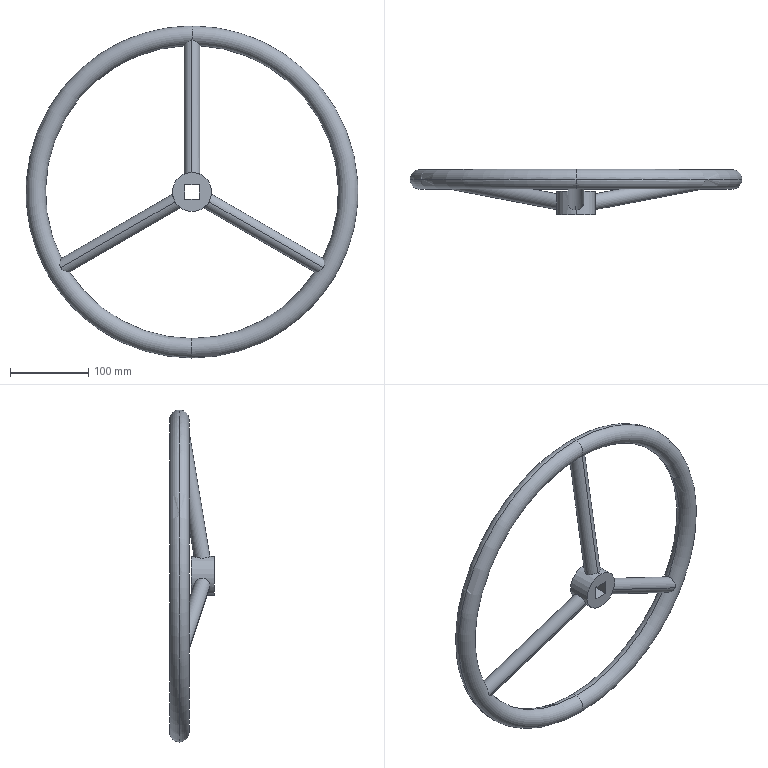Part | SolidWorks | features MirrorStock 1 | 1 solid | 22 faces | box 425 x 57.5 x 425 mm | volume 466638 mm3 | torus 8 | cylinder 8 | plane 6 | commonest cylinder face diameters 20 x6 50 x2